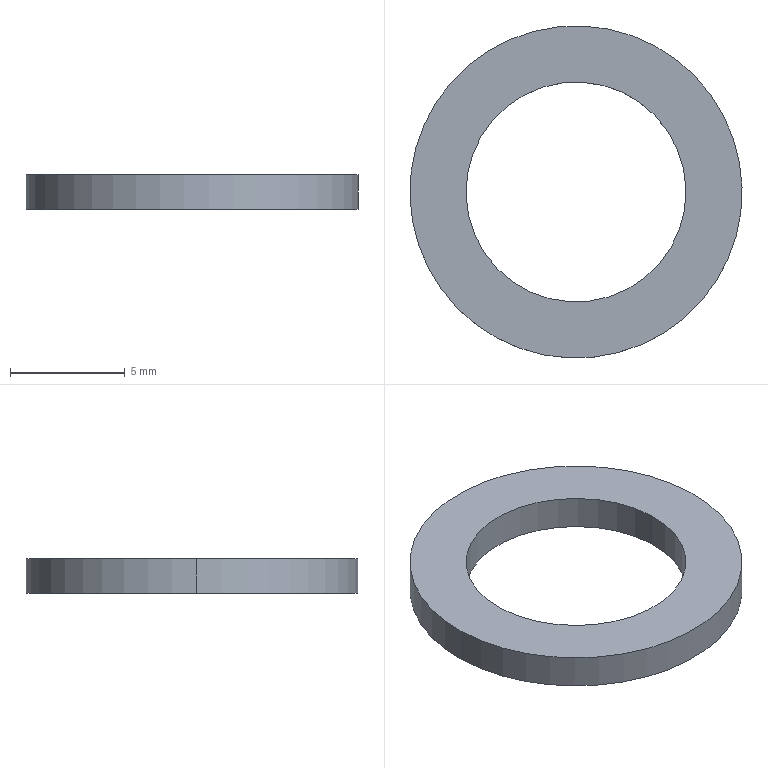Part | SolidWorks | features BaseBody 1 | 1 solid | 6 faces | box 14.5 x 14.5 x 1.5 mm | volume 139.122 mm3 | cylinder 4 | plane 2 | commonest cylinder face diameters 9.6 x2 14.5 x2
STEP:
#1=CARTESIAN_POINT('',(167.702,-0.1402,57.15));
#2=VERTEX_POINT('',#1);
#3=CARTESIAN_POINT('',(177.298,0.1402,57.15));
#4=VERTEX_POINT('',#3);
#5=CARTESIAN_POINT('',(172.5,0.,57.15));
#6=DIRECTION('',(0.,0.,1.));
#7=DIRECTION('',(0.9996,0.02921,0.));
#8=AXIS2_PLACEMENT_3D('',#5,#6,#7);
#9=CIRCLE('',#8,4.8);
#10=EDGE_CURVE('',#2,#4,#9,.T.);
#11=ORIENTED_EDGE('',*,*,#10,.T.);
#12=CARTESIAN_POINT('',(177.298,0.1402,55.65));
#13=VERTEX_POINT('',#12);
#14=CARTESIAN_POINT('',(177.298,0.1402,57.15));
#15=DIRECTION('',(0.,0.,-1.));
#16=VECTOR('',#15,1000.);
#17=LINE('',#14,#16);
#18=EDGE_CURVE('',#4,#13,#17,.T.);
#19=ORIENTED_EDGE('',*,*,#18,.T.);
#20=CARTESIAN_POINT('',(167.702,-0.1402,55.65));
#21=VERTEX_POINT('',#20);
#22=CARTESIAN_POINT('',(172.5,0.,55.65));
#23=DIRECTION('',(0.,0.,1.));
#24=DIRECTION('',(0.9996,0.02921,0.));
#25=AXIS2_PLACEMENT_3D('',#22,#23,#24);
#26=CIRCLE('',#25,4.8);
#27=EDGE_CURVE('',#21,#13,#26,.T.);
#28=ORIENTED_EDGE('',*,*,#27,.F.);
#29=CARTESIAN_POINT('',(167.702,-0.1402,57.15));
#30=DIRECTION('',(0.,0.,-1.));
#31=VECTOR('',#30,1000.);
#32=LINE('',#29,#31);
#33=EDGE_CURVE('',#2,#21,#32,.T.);
#34=ORIENTED_EDGE('',*,*,#33,.F.);
#35=EDGE_LOOP('',(#11,#19,#28,#34));
#36=FACE_OUTER_BOUND('',#35,.T.);
#37=CARTESIAN_POINT('',(172.5,0.,57.15));
#38=DIRECTION('',(0.,0.,-1.));
#39=DIRECTION('',(-0.9996,-0.02921,0.));
#40=AXIS2_PLACEMENT_3D('',#37,#38,#39);
#41=CYLINDRICAL_SURFACE('',#40,4.8);
#42=ADVANCED_FACE('',(#36),#41,.F.);
#43=CARTESIAN_POINT('',(179.747,0.2117,57.15));
#44=VERTEX_POINT('',#43);
#45=CARTESIAN_POINT('',(165.253,-0.2117,57.15));
#46=VERTEX_POINT('',#45);
#47=CARTESIAN_POINT('',(172.5,0.,57.15));
#48=DIRECTION('',(0.,0.,1.));
#49=DIRECTION('',(0.9996,0.02921,0.));
#50=AXIS2_PLACEMENT_3D('',#47,#48,#49);
#51=CIRCLE('',#50,7.25);
#52=EDGE_CURVE('',#44,#46,#51,.T.);
#53=ORIENTED_EDGE('',*,*,#52,.F.);
#54=CARTESIAN_POINT('',(179.747,0.2117,55.65));
#55=VERTEX_POINT('',#54);
#56=CARTESIAN_POINT('',(179.747,0.2117,57.15));
#57=DIRECTION('',(0.,0.,-1.));
#58=VECTOR('',#57,1000.);
#59=LINE('',#56,#58);
#60=EDGE_CURVE('',#44,#55,#59,.T.);
#61=ORIENTED_EDGE('',*,*,#60,.T.);
#62=CARTESIAN_POINT('',(165.253,-0.2117,55.65));
#63=VERTEX_POINT('',#62);
#64=CARTESIAN_POINT('',(172.5,0.,55.65));
#65=DIRECTION('',(0.,0.,1.));
#66=DIRECTION('',(0.9996,0.02921,0.));
#67=AXIS2_PLACEMENT_3D('',#64,#65,#66);
#68=CIRCLE('',#67,7.25);
#69=EDGE_CURVE('',#55,#63,#68,.T.);
#70=ORIENTED_EDGE('',*,*,#69,.T.);
#71=CARTESIAN_POINT('',(165.253,-0.2117,57.15));
#72=DIRECTION('',(0.,0.,-1.));
#73=VECTOR('',#72,1000.);
#74=LINE('',#71,#73);
#75=EDGE_CURVE('',#46,#63,#74,.T.);
#76=ORIENTED_EDGE('',*,*,#75,.F.);
#77=EDGE_LOOP('',(#53,#61,#70,#76));
#78=FACE_OUTER_BOUND('',#77,.T.);
#79=CARTESIAN_POINT('',(172.5,0.,57.15));
#80=DIRECTION('',(0.,0.,-1.));
#81=DIRECTION('',(-0.9996,-0.02921,0.));
#82=AXIS2_PLACEMENT_3D('',#79,#80,#81);
#83=CYLINDRICAL_SURFACE('',#82,7.25);
#84=ADVANCED_FACE('',(#78),#83,.T.);
#85=CARTESIAN_POINT('',(172.5,0.,57.15));
#86=DIRECTION('',(0.,0.,1.));
#87=DIRECTION('',(0.9996,0.02921,0.));
#88=AXIS2_PLACEMENT_3D('',#85,#86,#87);
#89=CIRCLE('',#88,7.25);
#90=EDGE_CURVE('',#46,#44,#89,.T.);
#91=ORIENTED_EDGE('',*,*,#90,.T.);
#92=ORIENTED_EDGE('',*,*,#52,.T.);
#93=EDGE_LOOP('',(#91,#92));
#94=FACE_OUTER_BOUND('',#93,.T.);
#95=ORIENTED_EDGE('',*,*,#10,.F.);
#96=CARTESIAN_POINT('',(172.5,0.,57.15));
#97=DIRECTION('',(0.,0.,1.));
#98=DIRECTION('',(0.9996,0.02921,0.));
#99=AXIS2_PLACEMENT_3D('',#96,#97,#98);
#100=CIRCLE('',#99,4.8);
#101=EDGE_CURVE('',#4,#2,#100,.T.);
#102=ORIENTED_EDGE('',*,*,#101,.F.);
#103=EDGE_LOOP('',(#95,#102));
#104=FACE_BOUND('',#103,.T.);
#105=CARTESIAN_POINT('',(172.5,0.,57.15));
#106=DIRECTION('',(0.,0.,1.));
#107=DIRECTION('',(0.9996,0.02921,0.));
#108=AXIS2_PLACEMENT_3D('',#105,#106,#107);
#109=PLANE('',#108);
#110=ADVANCED_FACE('',(#94,#104),#109,.T.);
#111=CARTESIAN_POINT('',(172.5,0.,55.65));
#112=DIRECTION('',(0.,0.,1.));
#113=DIRECTION('',(0.9996,0.02921,0.));
#114=AXIS2_PLACEMENT_3D('',#111,#112,#113);
#115=CIRCLE('',#114,7.25);
#116=EDGE_CURVE('',#63,#55,#115,.T.);
#117=ORIENTED_EDGE('',*,*,#116,.F.);
#118=ORIENTED_EDGE('',*,*,#69,.F.);
#119=EDGE_LOOP('',(#117,#118));
#120=FACE_OUTER_BOUND('',#119,.T.);
#121=ORIENTED_EDGE('',*,*,#27,.T.);
#122=CARTESIAN_POINT('',(172.5,0.,55.65));
#123=DIRECTION('',(0.,0.,1.));
#124=DIRECTION('',(0.9996,0.02921,0.));
#125=AXIS2_PLACEMENT_3D('',#122,#123,#124);
#126=CIRCLE('',#125,4.8);
#127=EDGE_CURVE('',#13,#21,#126,.T.);
#128=ORIENTED_EDGE('',*,*,#127,.T.);
#129=EDGE_LOOP('',(#121,#128));
#130=FACE_BOUND('',#129,.T.);
#131=CARTESIAN_POINT('',(172.5,0.,55.65));
#132=DIRECTION('',(0.,0.,1.));
#133=DIRECTION('',(0.9996,0.02921,0.));
#134=AXIS2_PLACEMENT_3D('',#131,#132,#133);
#135=PLANE('',#134);
#136=ADVANCED_FACE('',(#120,#130),#135,.F.);
#137=ORIENTED_EDGE('',*,*,#60,.F.);
#138=ORIENTED_EDGE('',*,*,#90,.F.);
#139=ORIENTED_EDGE('',*,*,#75,.T.);
#140=ORIENTED_EDGE('',*,*,#116,.T.);
#141=EDGE_LOOP('',(#137,#138,#139,#140));
#142=FACE_OUTER_BOUND('',#141,.T.);
#143=CARTESIAN_POINT('',(172.5,0.,57.15));
#144=DIRECTION('',(0.,0.,-1.));
#145=DIRECTION('',(-0.9996,-0.02921,0.));
#146=AXIS2_PLACEMENT_3D('',#143,#144,#145);
#147=CYLINDRICAL_SURFACE('',#146,7.25);
#148=ADVANCED_FACE('',(#142),#147,.T.);
#149=ORIENTED_EDGE('',*,*,#18,.F.);
#150=ORIENTED_EDGE('',*,*,#101,.T.);
#151=ORIENTED_EDGE('',*,*,#33,.T.);
#152=ORIENTED_EDGE('',*,*,#127,.F.);
#153=EDGE_LOOP('',(#149,#150,#151,#152));
#154=FACE_OUTER_BOUND('',#153,.T.);
#155=CARTESIAN_POINT('',(172.5,0.,57.15));
#156=DIRECTION('',(0.,0.,-1.));
#157=DIRECTION('',(-0.9996,-0.02921,0.));
#158=AXIS2_PLACEMENT_3D('',#155,#156,#157);
#159=CYLINDRICAL_SURFACE('',#158,4.8);
#160=ADVANCED_FACE('',(#154),#159,.F.);
#161=CLOSED_SHELL('',(#42,#84,#110,#136,#148,#160));
#162=MANIFOLD_SOLID_BREP('',#161);
#163=CARTESIAN_POINT('',(0.,0.,0.));
#164=DIRECTION('',(0.,0.,1.));
#165=DIRECTION('',(1.,0.,0.));
#166=AXIS2_PLACEMENT_3D('',#163,#164,#165);
#167=(LENGTH_UNIT()NAMED_UNIT(*)SI_UNIT(.MILLI.,.METRE.));
#168=UNCERTAINTY_MEASURE_WITH_UNIT(LENGTH_MEASURE(0.00001),#167,'','');
#169=(NAMED_UNIT(*)PLANE_ANGLE_UNIT()SI_UNIT($,.RADIAN.));
#170=(NAMED_UNIT(*)SI_UNIT($,.STERADIAN.)SOLID_ANGLE_UNIT());
#171=(GEOMETRIC_REPRESENTATION_CONTEXT(3)GLOBAL_UNCERTAINTY_ASSIGNED_CONTEXT((#168))GLOBAL_UNIT_ASSIGNED_CONTEXT((#167,#169,#170))REPRESENTATION_CONTEXT('',''));
#172=ADVANCED_BREP_SHAPE_REPRESENTATION('',(#162,#166),#171);